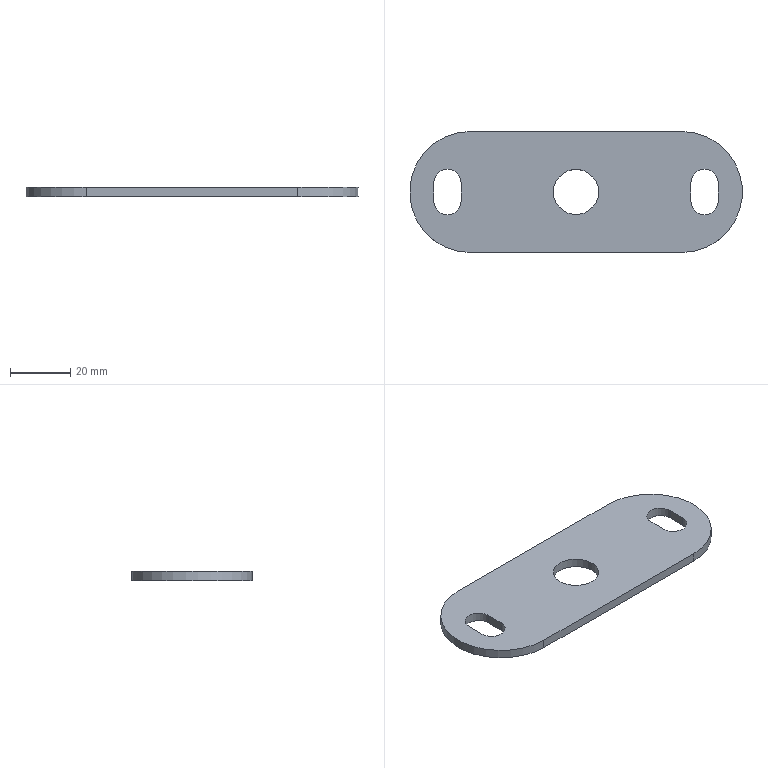Part | STEP file | PN_0011_default | 1 solid | 15 faces | box 110 x 40 x 3 mm | volume 10934 mm3 | plane 8 | cylinder 7 | commonest cylinder face diameters 9 x4 40 x2 15 x1
STEP:
#1=CARTESIAN_POINT('',(0.,0.,0.));
#2=DIRECTION('',(0.,0.,1.));
#3=DIRECTION('',(1.,0.,0.));
#4=AXIS2_PLACEMENT_3D('',#1,#2,#3);
#5=CARTESIAN_POINT('',(7.5,0.,3.));
#6=VERTEX_POINT('',#5);
#7=CARTESIAN_POINT('',(0.,0.,3.));
#8=DIRECTION('',(0.,0.,1.));
#9=DIRECTION('',(1.,0.,0.));
#10=AXIS2_PLACEMENT_3D('',#7,#8,#9);
#11=CIRCLE('',#10,7.5);
#12=CARTESIAN_POINT('',(-35.,0.,3.));
#13=DIRECTION('',(0.,0.,1.));
#14=DIRECTION('',(1.,0.,0.));
#15=AXIS2_PLACEMENT_3D('',#12,#13,#14);
#16=PLANE('',#15);
#17=CARTESIAN_POINT('',(35.,0.));
#18=DIRECTION('',(1.,0.));
#19=AXIS2_PLACEMENT_2D('',#17,#18);
#20=CIRCLE('',#19,7.5);
#21=(GEOMETRIC_REPRESENTATION_CONTEXT(2)PARAMETRIC_REPRESENTATION_CONTEXT()REPRESENTATION_CONTEXT('',''));
#22=DEFINITIONAL_REPRESENTATION('',(#20),#21);
#23=PCURVE('',#16,#22);
#24=CARTESIAN_POINT('',(0.,0.,-7.));
#25=DIRECTION('',(0.,0.,1.));
#26=DIRECTION('',(1.,0.,0.));
#27=AXIS2_PLACEMENT_3D('',#24,#25,#26);
#28=CYLINDRICAL_SURFACE('',#27,7.5);
#29=CARTESIAN_POINT('',(0.,10.));
#30=DIRECTION('',(1.,0.));
#31=VECTOR('',#30,1.);
#32=LINE('',#29,#31);
#33=(GEOMETRIC_REPRESENTATION_CONTEXT(2)PARAMETRIC_REPRESENTATION_CONTEXT()REPRESENTATION_CONTEXT('',''));
#34=DEFINITIONAL_REPRESENTATION('',(#32),#33);
#35=PCURVE('',#28,#34);
#36=SURFACE_CURVE('',#11,(#23,#35),.PCURVE_S1.);
#37=EDGE_CURVE('',#6,#6,#36,.T.);
#38=ORIENTED_EDGE('',*,*,#37,.F.);
#39=EDGE_LOOP('',(#38));
#40=FACE_BOUND('',#39,.T.);
#41=CARTESIAN_POINT('',(-47.,3.,3.));
#42=VERTEX_POINT('',#41);
#43=CARTESIAN_POINT('',(-47.,-3.,3.));
#44=VERTEX_POINT('',#43);
#45=CARTESIAN_POINT('',(-47.,3.,3.));
#46=DIRECTION('',(0.,-1.,0.));
#47=VECTOR('',#46,1.);
#48=LINE('',#45,#47);
#49=CARTESIAN_POINT('',(-12.,3.));
#50=DIRECTION('',(0.,-1.));
#51=VECTOR('',#50,1.);
#52=LINE('',#49,#51);
#53=(GEOMETRIC_REPRESENTATION_CONTEXT(2)PARAMETRIC_REPRESENTATION_CONTEXT()REPRESENTATION_CONTEXT('',''));
#54=DEFINITIONAL_REPRESENTATION('',(#52),#53);
#55=PCURVE('',#16,#54);
#56=CARTESIAN_POINT('',(-47.,3.,3.));
#57=DIRECTION('',(1.,0.,0.));
#58=DIRECTION('',(0.,0.,-1.));
#59=AXIS2_PLACEMENT_3D('',#56,#57,#58);
#60=PLANE('',#59);
#61=CARTESIAN_POINT('',(0.,0.));
#62=DIRECTION('',(0.,-1.));
#63=VECTOR('',#62,1.);
#64=LINE('',#61,#63);
#65=(GEOMETRIC_REPRESENTATION_CONTEXT(2)PARAMETRIC_REPRESENTATION_CONTEXT()REPRESENTATION_CONTEXT('',''));
#66=DEFINITIONAL_REPRESENTATION('',(#64),#65);
#67=PCURVE('',#60,#66);
#68=SURFACE_CURVE('',#48,(#55,#67),.PCURVE_S1.);
#69=EDGE_CURVE('',#42,#44,#68,.T.);
#70=ORIENTED_EDGE('',*,*,#69,.F.);
#71=CARTESIAN_POINT('',(-38.,3.,3.));
#72=VERTEX_POINT('',#71);
#73=CARTESIAN_POINT('',(-42.5,3.,3.));
#74=DIRECTION('',(0.,0.,1.));
#75=DIRECTION('',(1.,0.,0.));
#76=AXIS2_PLACEMENT_3D('',#73,#74,#75);
#77=CIRCLE('',#76,4.5);
#78=CARTESIAN_POINT('',(-7.5,3.));
#79=DIRECTION('',(1.,0.));
#80=AXIS2_PLACEMENT_2D('',#78,#79);
#81=CIRCLE('',#80,4.5);
#82=(GEOMETRIC_REPRESENTATION_CONTEXT(2)PARAMETRIC_REPRESENTATION_CONTEXT()REPRESENTATION_CONTEXT('',''));
#83=DEFINITIONAL_REPRESENTATION('',(#81),#82);
#84=PCURVE('',#16,#83);
#85=CARTESIAN_POINT('',(-42.5,3.,3.));
#86=DIRECTION('',(0.,0.,-1.));
#87=DIRECTION('',(-1.,0.,0.));
#88=AXIS2_PLACEMENT_3D('',#85,#86,#87);
#89=CYLINDRICAL_SURFACE('',#88,4.5);
#90=CARTESIAN_POINT('',(3.142,0.));
#91=DIRECTION('',(-1.,0.));
#92=VECTOR('',#91,1.);
#93=LINE('',#90,#92);
#94=(GEOMETRIC_REPRESENTATION_CONTEXT(2)PARAMETRIC_REPRESENTATION_CONTEXT()REPRESENTATION_CONTEXT('',''));
#95=DEFINITIONAL_REPRESENTATION('',(#93),#94);
#96=PCURVE('',#89,#95);
#97=SURFACE_CURVE('',#77,(#84,#96),.PCURVE_S1.);
#98=EDGE_CURVE('',#72,#42,#97,.T.);
#99=ORIENTED_EDGE('',*,*,#98,.F.);
#100=CARTESIAN_POINT('',(-38.,-3.,3.));
#101=VERTEX_POINT('',#100);
#102=CARTESIAN_POINT('',(-38.,3.,3.));
#103=DIRECTION('',(0.,1.,0.));
#104=VECTOR('',#103,1.);
#105=LINE('',#102,#104);
#106=CARTESIAN_POINT('',(-3.,3.));
#107=DIRECTION('',(0.,1.));
#108=VECTOR('',#107,1.);
#109=LINE('',#106,#108);
#110=(GEOMETRIC_REPRESENTATION_CONTEXT(2)PARAMETRIC_REPRESENTATION_CONTEXT()REPRESENTATION_CONTEXT('',''));
#111=DEFINITIONAL_REPRESENTATION('',(#109),#110);
#112=PCURVE('',#16,#111);
#113=CARTESIAN_POINT('',(-38.,3.,3.));
#114=DIRECTION('',(-1.,0.,0.));
#115=DIRECTION('',(0.,0.,1.));
#116=AXIS2_PLACEMENT_3D('',#113,#114,#115);
#117=PLANE('',#116);
#118=CARTESIAN_POINT('',(0.,0.));
#119=DIRECTION('',(0.,1.));
#120=VECTOR('',#119,1.);
#121=LINE('',#118,#120);
#122=(GEOMETRIC_REPRESENTATION_CONTEXT(2)PARAMETRIC_REPRESENTATION_CONTEXT()REPRESENTATION_CONTEXT('',''));
#123=DEFINITIONAL_REPRESENTATION('',(#121),#122);
#124=PCURVE('',#117,#123);
#125=SURFACE_CURVE('',#105,(#112,#124),.PCURVE_S1.);
#126=EDGE_CURVE('',#101,#72,#125,.T.);
#127=ORIENTED_EDGE('',*,*,#126,.F.);
#128=CARTESIAN_POINT('',(-42.5,-3.,3.));
#129=DIRECTION('',(0.,0.,1.));
#130=DIRECTION('',(1.,0.,0.));
#131=AXIS2_PLACEMENT_3D('',#128,#129,#130);
#132=CIRCLE('',#131,4.5);
#133=CARTESIAN_POINT('',(-7.5,-3.));
#134=DIRECTION('',(1.,0.));
#135=AXIS2_PLACEMENT_2D('',#133,#134);
#136=CIRCLE('',#135,4.5);
#137=(GEOMETRIC_REPRESENTATION_CONTEXT(2)PARAMETRIC_REPRESENTATION_CONTEXT()REPRESENTATION_CONTEXT('',''));
#138=DEFINITIONAL_REPRESENTATION('',(#136),#137);
#139=PCURVE('',#16,#138);
#140=CARTESIAN_POINT('',(-42.5,-3.,3.));
#141=DIRECTION('',(0.,0.,-1.));
#142=DIRECTION('',(-1.,0.,0.));
#143=AXIS2_PLACEMENT_3D('',#140,#141,#142);
#144=CYLINDRICAL_SURFACE('',#143,4.5);
#145=CARTESIAN_POINT('',(9.425,0.));
#146=DIRECTION('',(-1.,0.));
#147=VECTOR('',#146,1.);
#148=LINE('',#145,#147);
#149=(GEOMETRIC_REPRESENTATION_CONTEXT(2)PARAMETRIC_REPRESENTATION_CONTEXT()REPRESENTATION_CONTEXT('',''));
#150=DEFINITIONAL_REPRESENTATION('',(#148),#149);
#151=PCURVE('',#144,#150);
#152=SURFACE_CURVE('',#132,(#139,#151),.PCURVE_S1.);
#153=EDGE_CURVE('',#44,#101,#152,.T.);
#154=ORIENTED_EDGE('',*,*,#153,.F.);
#155=EDGE_LOOP('',(#70,#99,#127,#154));
#156=FACE_BOUND('',#155,.T.);
#157=CARTESIAN_POINT('',(-35.,20.,3.));
#158=VERTEX_POINT('',#157);
#159=CARTESIAN_POINT('',(-35.,-20.,3.));
#160=VERTEX_POINT('',#159);
#161=CARTESIAN_POINT('',(-35.,0.,3.));
#162=DIRECTION('',(0.,0.,1.));
#163=DIRECTION('',(1.,0.,0.));
#164=AXIS2_PLACEMENT_3D('',#161,#162,#163);
#165=CIRCLE('',#164,20.);
#166=CARTESIAN_POINT('',(0.,0.));
#167=DIRECTION('',(1.,0.));
#168=AXIS2_PLACEMENT_2D('',#166,#167);
#169=CIRCLE('',#168,20.);
#170=(GEOMETRIC_REPRESENTATION_CONTEXT(2)PARAMETRIC_REPRESENTATION_CONTEXT()REPRESENTATION_CONTEXT('',''));
#171=DEFINITIONAL_REPRESENTATION('',(#169),#170);
#172=PCURVE('',#16,#171);
#173=CARTESIAN_POINT('',(-35.,0.,3.));
#174=DIRECTION('',(0.,0.,-1.));
#175=DIRECTION('',(-1.,0.,0.));
#176=AXIS2_PLACEMENT_3D('',#173,#174,#175);
#177=CYLINDRICAL_SURFACE('',#176,20.);
#178=CARTESIAN_POINT('',(3.142,0.));
#179=DIRECTION('',(-1.,0.));
#180=VECTOR('',#179,1.);
#181=LINE('',#178,#180);
#182=(GEOMETRIC_REPRESENTATION_CONTEXT(2)PARAMETRIC_REPRESENTATION_CONTEXT()REPRESENTATION_CONTEXT('',''));
#183=DEFINITIONAL_REPRESENTATION('',(#181),#182);
#184=PCURVE('',#177,#183);
#185=SURFACE_CURVE('',#165,(#172,#184),.PCURVE_S1.);
#186=EDGE_CURVE('',#158,#160,#185,.T.);
#187=ORIENTED_EDGE('',*,*,#186,.T.);
#188=CARTESIAN_POINT('',(35.,-20.,3.));
#189=VERTEX_POINT('',#188);
#190=CARTESIAN_POINT('',(-35.,-20.,3.));
#191=DIRECTION('',(1.,0.,0.));
#192=VECTOR('',#191,1.);
#193=LINE('',#190,#192);
#194=CARTESIAN_POINT('',(0.,-20.));
#195=DIRECTION('',(1.,0.));
#196=VECTOR('',#195,1.);
#197=LINE('',#194,#196);
#198=(GEOMETRIC_REPRESENTATION_CONTEXT(2)PARAMETRIC_REPRESENTATION_CONTEXT()REPRESENTATION_CONTEXT('',''));
#199=DEFINITIONAL_REPRESENTATION('',(#197),#198);
#200=PCURVE('',#16,#199);
#201=CARTESIAN_POINT('',(-35.,-20.,3.));
#202=DIRECTION('',(0.,1.,0.));
#203=DIRECTION('',(0.,0.,1.));
#204=AXIS2_PLACEMENT_3D('',#201,#202,#203);
#205=PLANE('',#204);
#206=CARTESIAN_POINT('',(0.,0.));
#207=DIRECTION('',(0.,1.));
#208=VECTOR('',#207,1.);
#209=LINE('',#206,#208);
#210=(GEOMETRIC_REPRESENTATION_CONTEXT(2)PARAMETRIC_REPRESENTATION_CONTEXT()REPRESENTATION_CONTEXT('',''));
#211=DEFINITIONAL_REPRESENTATION('',(#209),#210);
#212=PCURVE('',#205,#211);
#213=SURFACE_CURVE('',#193,(#200,#212),.PCURVE_S1.);
#214=EDGE_CURVE('',#160,#189,#213,.T.);
#215=ORIENTED_EDGE('',*,*,#214,.T.);
#216=CARTESIAN_POINT('',(35.,20.,3.));
#217=VERTEX_POINT('',#216);
#218=CARTESIAN_POINT('',(35.,0.,3.));
#219=DIRECTION('',(0.,0.,1.));
#220=DIRECTION('',(-1.,0.,0.));
#221=AXIS2_PLACEMENT_3D('',#218,#219,#220);
#222=CIRCLE('',#221,20.);
#223=CARTESIAN_POINT('',(70.,0.));
#224=DIRECTION('',(-1.,0.));
#225=AXIS2_PLACEMENT_2D('',#223,#224);
#226=CIRCLE('',#225,20.);
#227=(GEOMETRIC_REPRESENTATION_CONTEXT(2)PARAMETRIC_REPRESENTATION_CONTEXT()REPRESENTATION_CONTEXT('',''));
#228=DEFINITIONAL_REPRESENTATION('',(#226),#227);
#229=PCURVE('',#16,#228);
#230=CARTESIAN_POINT('',(35.,0.,3.));
#231=DIRECTION('',(0.,0.,-1.));
#232=DIRECTION('',(-1.,0.,0.));
#233=AXIS2_PLACEMENT_3D('',#230,#231,#232);
#234=CYLINDRICAL_SURFACE('',#233,20.);
#235=CARTESIAN_POINT('',(6.283,0.));
#236=DIRECTION('',(-1.,0.));
#237=VECTOR('',#236,1.);
#238=LINE('',#235,#237);
#239=(GEOMETRIC_REPRESENTATION_CONTEXT(2)PARAMETRIC_REPRESENTATION_CONTEXT()REPRESENTATION_CONTEXT('',''));
#240=DEFINITIONAL_REPRESENTATION('',(#238),#239);
#241=PCURVE('',#234,#240);
#242=SURFACE_CURVE('',#222,(#229,#241),.PCURVE_S1.);
#243=EDGE_CURVE('',#189,#217,#242,.T.);
#244=ORIENTED_EDGE('',*,*,#243,.T.);
#245=CARTESIAN_POINT('',(-35.,20.,3.));
#246=DIRECTION('',(-1.,0.,0.));
#247=VECTOR('',#246,1.);
#248=LINE('',#245,#247);
#249=CARTESIAN_POINT('',(0.,20.));
#250=DIRECTION('',(-1.,0.));
#251=VECTOR('',#250,1.);
#252=LINE('',#249,#251);
#253=(GEOMETRIC_REPRESENTATION_CONTEXT(2)PARAMETRIC_REPRESENTATION_CONTEXT()REPRESENTATION_CONTEXT('',''));
#254=DEFINITIONAL_REPRESENTATION('',(#252),#253);
#255=PCURVE('',#16,#254);
#256=CARTESIAN_POINT('',(-35.,20.,3.));
#257=DIRECTION('',(0.,-1.,0.));
#258=DIRECTION('',(0.,0.,-1.));
#259=AXIS2_PLACEMENT_3D('',#256,#257,#258);
#260=PLANE('',#259);
#261=CARTESIAN_POINT('',(0.,0.));
#262=DIRECTION('',(0.,-1.));
#263=VECTOR('',#262,1.);
#264=LINE('',#261,#263);
#265=(GEOMETRIC_REPRESENTATION_CONTEXT(2)PARAMETRIC_REPRESENTATION_CONTEXT()REPRESENTATION_CONTEXT('',''));
#266=DEFINITIONAL_REPRESENTATION('',(#264),#265);
#267=PCURVE('',#260,#266);
#268=SURFACE_CURVE('',#248,(#255,#267),.PCURVE_S1.);
#269=EDGE_CURVE('',#217,#158,#268,.T.);
#270=ORIENTED_EDGE('',*,*,#269,.T.);
#271=EDGE_LOOP('',(#187,#215,#244,#270));
#272=FACE_BOUND('',#271,.T.);
#273=CARTESIAN_POINT('',(47.,-3.,3.));
#274=VERTEX_POINT('',#273);
#275=CARTESIAN_POINT('',(47.,3.,3.));
#276=VERTEX_POINT('',#275);
#277=CARTESIAN_POINT('',(47.,3.,3.));
#278=DIRECTION('',(0.,1.,0.));
#279=VECTOR('',#278,1.);
#280=LINE('',#277,#279);
#281=CARTESIAN_POINT('',(82.,3.));
#282=DIRECTION('',(0.,1.));
#283=VECTOR('',#282,1.);
#284=LINE('',#281,#283);
#285=(GEOMETRIC_REPRESENTATION_CONTEXT(2)PARAMETRIC_REPRESENTATION_CONTEXT()REPRESENTATION_CONTEXT('',''));
#286=DEFINITIONAL_REPRESENTATION('',(#284),#285);
#287=PCURVE('',#16,#286);
#288=CARTESIAN_POINT('',(47.,3.,3.));
#289=DIRECTION('',(-1.,0.,0.));
#290=DIRECTION('',(0.,0.,1.));
#291=AXIS2_PLACEMENT_3D('',#288,#289,#290);
#292=PLANE('',#291);
#293=CARTESIAN_POINT('',(0.,0.));
#294=DIRECTION('',(0.,1.));
#295=VECTOR('',#294,1.);
#296=LINE('',#293,#295);
#297=(GEOMETRIC_REPRESENTATION_CONTEXT(2)PARAMETRIC_REPRESENTATION_CONTEXT()REPRESENTATION_CONTEXT('',''));
#298=DEFINITIONAL_REPRESENTATION('',(#296),#297);
#299=PCURVE('',#292,#298);
#300=SURFACE_CURVE('',#280,(#287,#299),.PCURVE_S1.);
#301=EDGE_CURVE('',#274,#276,#300,.T.);
#302=ORIENTED_EDGE('',*,*,#301,.F.);
#303=CARTESIAN_POINT('',(38.,-3.,3.));
#304=VERTEX_POINT('',#303);
#305=CARTESIAN_POINT('',(42.5,-3.,3.));
#306=DIRECTION('',(0.,0.,1.));
#307=DIRECTION('',(1.,0.,0.));
#308=AXIS2_PLACEMENT_3D('',#305,#306,#307);
#309=CIRCLE('',#308,4.5);
#310=CARTESIAN_POINT('',(77.5,-3.));
#311=DIRECTION('',(1.,0.));
#312=AXIS2_PLACEMENT_2D('',#310,#311);
#313=CIRCLE('',#312,4.5);
#314=(GEOMETRIC_REPRESENTATION_CONTEXT(2)PARAMETRIC_REPRESENTATION_CONTEXT()REPRESENTATION_CONTEXT('',''));
#315=DEFINITIONAL_REPRESENTATION('',(#313),#314);
#316=PCURVE('',#16,#315);
#317=CARTESIAN_POINT('',(42.5,-3.,3.));
#318=DIRECTION('',(0.,0.,-1.));
#319=DIRECTION('',(-1.,0.,0.));
#320=AXIS2_PLACEMENT_3D('',#317,#318,#319);
#321=CYLINDRICAL_SURFACE('',#320,4.5);
#322=CARTESIAN_POINT('',(9.425,0.));
#323=DIRECTION('',(-1.,0.));
#324=VECTOR('',#323,1.);
#325=LINE('',#322,#324);
#326=(GEOMETRIC_REPRESENTATION_CONTEXT(2)PARAMETRIC_REPRESENTATION_CONTEXT()REPRESENTATION_CONTEXT('',''));
#327=DEFINITIONAL_REPRESENTATION('',(#325),#326);
#328=PCURVE('',#321,#327);
#329=SURFACE_CURVE('',#309,(#316,#328),.PCURVE_S1.);
#330=EDGE_CURVE('',#304,#274,#329,.T.);
#331=ORIENTED_EDGE('',*,*,#330,.F.);
#332=CARTESIAN_POINT('',(38.,3.,3.));
#333=VERTEX_POINT('',#332);
#334=CARTESIAN_POINT('',(38.,3.,3.));
#335=DIRECTION('',(0.,-1.,0.));
#336=VECTOR('',#335,1.);
#337=LINE('',#334,#336);
#338=CARTESIAN_POINT('',(73.,3.));
#339=DIRECTION('',(0.,-1.));
#340=VECTOR('',#339,1.);
#341=LINE('',#338,#340);
#342=(GEOMETRIC_REPRESENTATION_CONTEXT(2)PARAMETRIC_REPRESENTATION_CONTEXT()REPRESENTATION_CONTEXT('',''));
#343=DEFINITIONAL_REPRESENTATION('',(#341),#342);
#344=PCURVE('',#16,#343);
#345=CARTESIAN_POINT('',(38.,3.,3.));
#346=DIRECTION('',(1.,0.,0.));
#347=DIRECTION('',(0.,0.,-1.));
#348=AXIS2_PLACEMENT_3D('',#345,#346,#347);
#349=PLANE('',#348);
#350=CARTESIAN_POINT('',(0.,0.));
#351=DIRECTION('',(0.,-1.));
#352=VECTOR('',#351,1.);
#353=LINE('',#350,#352);
#354=(GEOMETRIC_REPRESENTATION_CONTEXT(2)PARAMETRIC_REPRESENTATION_CONTEXT()REPRESENTATION_CONTEXT('',''));
#355=DEFINITIONAL_REPRESENTATION('',(#353),#354);
#356=PCURVE('',#349,#355);
#357=SURFACE_CURVE('',#337,(#344,#356),.PCURVE_S1.);
#358=EDGE_CURVE('',#333,#304,#357,.T.);
#359=ORIENTED_EDGE('',*,*,#358,.F.);
#360=CARTESIAN_POINT('',(42.5,3.,3.));
#361=DIRECTION('',(0.,0.,1.));
#362=DIRECTION('',(1.,0.,0.));
#363=AXIS2_PLACEMENT_3D('',#360,#361,#362);
#364=CIRCLE('',#363,4.5);
#365=CARTESIAN_POINT('',(77.5,3.));
#366=DIRECTION('',(1.,0.));
#367=AXIS2_PLACEMENT_2D('',#365,#366);
#368=CIRCLE('',#367,4.5);
#369=(GEOMETRIC_REPRESENTATION_CONTEXT(2)PARAMETRIC_REPRESENTATION_CONTEXT()REPRESENTATION_CONTEXT('',''));
#370=DEFINITIONAL_REPRESENTATION('',(#368),#369);
#371=PCURVE('',#16,#370);
#372=CARTESIAN_POINT('',(42.5,3.,3.));
#373=DIRECTION('',(0.,0.,-1.));
#374=DIRECTION('',(-1.,0.,0.));
#375=AXIS2_PLACEMENT_3D('',#372,#373,#374);
#376=CYLINDRICAL_SURFACE('',#375,4.5);
#377=CARTESIAN_POINT('',(3.142,0.));
#378=DIRECTION('',(-1.,0.));
#379=VECTOR('',#378,1.);
#380=LINE('',#377,#379);
#381=(GEOMETRIC_REPRESENTATION_CONTEXT(2)PARAMETRIC_REPRESENTATION_CONTEXT()REPRESENTATION_CONTEXT('',''));
#382=DEFINITIONAL_REPRESENTATION('',(#380),#381);
#383=PCURVE('',#376,#382);
#384=SURFACE_CURVE('',#364,(#371,#383),.PCURVE_S1.);
#385=EDGE_CURVE('',#276,#333,#384,.T.);
#386=ORIENTED_EDGE('',*,*,#385,.F.);
#387=EDGE_LOOP('',(#302,#331,#359,#386));
#388=FACE_BOUND('',#387,.T.);
#389=ADVANCED_FACE('',(#40,#156,#272,#388),#16,.T.);
#390=CARTESIAN_POINT('',(7.5,0.,0.));
#391=VERTEX_POINT('',#390);
#392=CARTESIAN_POINT('',(0.,0.,0.));
#393=DIRECTION('',(0.,0.,1.));
#394=DIRECTION('',(1.,0.,0.));
#395=AXIS2_PLACEMENT_3D('',#392,#393,#394);
#396=CIRCLE('',#395,7.5);
#397=CARTESIAN_POINT('',(-35.,0.,0.));
#398=DIRECTION('',(0.,0.,1.));
#399=DIRECTION('',(1.,0.,0.));
#400=AXIS2_PLACEMENT_3D('',#397,#398,#399);
#401=PLANE('',#400);
#402=CARTESIAN_POINT('',(35.,0.));
#403=DIRECTION('',(1.,0.));
#404=AXIS2_PLACEMENT_2D('',#402,#403);
#405=CIRCLE('',#404,7.5);
#406=(GEOMETRIC_REPRESENTATION_CONTEXT(2)PARAMETRIC_REPRESENTATION_CONTEXT()REPRESENTATION_CONTEXT('',''));
#407=DEFINITIONAL_REPRESENTATION('',(#405),#406);
#408=PCURVE('',#401,#407);
#409=CARTESIAN_POINT('',(0.,7.));
#410=DIRECTION('',(1.,0.));
#411=VECTOR('',#410,1.);
#412=LINE('',#409,#411);
#413=(GEOMETRIC_REPRESENTATION_CONTEXT(2)PARAMETRIC_REPRESENTATION_CONTEXT()REPRESENTATION_CONTEXT('',''));
#414=DEFINITIONAL_REPRESENTATION('',(#412),#413);
#415=PCURVE('',#28,#414);
#416=SURFACE_CURVE('',#396,(#408,#415),.PCURVE_S1.);
#417=EDGE_CURVE('',#391,#391,#416,.T.);
#418=ORIENTED_EDGE('',*,*,#417,.T.);
#419=EDGE_LOOP('',(#418));
#420=FACE_BOUND('',#419,.T.);
#421=CARTESIAN_POINT('',(-38.,3.,0.));
#422=VERTEX_POINT('',#421);
#423=CARTESIAN_POINT('',(-47.,3.,0.));
#424=VERTEX_POINT('',#423);
#425=CARTESIAN_POINT('',(-42.5,3.,0.));
#426=DIRECTION('',(0.,0.,1.));
#427=DIRECTION('',(1.,0.,0.));
#428=AXIS2_PLACEMENT_3D('',#425,#426,#427);
#429=CIRCLE('',#428,4.5);
#430=CARTESIAN_POINT('',(-7.5,3.));
#431=DIRECTION('',(1.,0.));
#432=AXIS2_PLACEMENT_2D('',#430,#431);
#433=CIRCLE('',#432,4.5);
#434=(GEOMETRIC_REPRESENTATION_CONTEXT(2)PARAMETRIC_REPRESENTATION_CONTEXT()REPRESENTATION_CONTEXT('',''));
#435=DEFINITIONAL_REPRESENTATION('',(#433),#434);
#436=PCURVE('',#401,#435);
#437=CARTESIAN_POINT('',(3.142,3.));
#438=DIRECTION('',(-1.,0.));
#439=VECTOR('',#438,1.);
#440=LINE('',#437,#439);
#441=(GEOMETRIC_REPRESENTATION_CONTEXT(2)PARAMETRIC_REPRESENTATION_CONTEXT()REPRESENTATION_CONTEXT('',''));
#442=DEFINITIONAL_REPRESENTATION('',(#440),#441);
#443=PCURVE('',#89,#442);
#444=SURFACE_CURVE('',#429,(#436,#443),.PCURVE_S1.);
#445=EDGE_CURVE('',#422,#424,#444,.T.);
#446=ORIENTED_EDGE('',*,*,#445,.T.);
#447=CARTESIAN_POINT('',(-47.,-3.,0.));
#448=VERTEX_POINT('',#447);
#449=CARTESIAN_POINT('',(-47.,3.,0.));
#450=DIRECTION('',(0.,-1.,0.));
#451=VECTOR('',#450,1.);
#452=LINE('',#449,#451);
#453=CARTESIAN_POINT('',(-12.,3.));
#454=DIRECTION('',(0.,-1.));
#455=VECTOR('',#454,1.);
#456=LINE('',#453,#455);
#457=(GEOMETRIC_REPRESENTATION_CONTEXT(2)PARAMETRIC_REPRESENTATION_CONTEXT()REPRESENTATION_CONTEXT('',''));
#458=DEFINITIONAL_REPRESENTATION('',(#456),#457);
#459=PCURVE('',#401,#458);
#460=CARTESIAN_POINT('',(3.,0.));
#461=DIRECTION('',(0.,-1.));
#462=VECTOR('',#461,1.);
#463=LINE('',#460,#462);
#464=(GEOMETRIC_REPRESENTATION_CONTEXT(2)PARAMETRIC_REPRESENTATION_CONTEXT()REPRESENTATION_CONTEXT('',''));
#465=DEFINITIONAL_REPRESENTATION('',(#463),#464);
#466=PCURVE('',#60,#465);
#467=SURFACE_CURVE('',#452,(#459,#466),.PCURVE_S1.);
#468=EDGE_CURVE('',#424,#448,#467,.T.);
#469=ORIENTED_EDGE('',*,*,#468,.T.);
#470=CARTESIAN_POINT('',(-38.,-3.,0.));
#471=VERTEX_POINT('',#470);
#472=CARTESIAN_POINT('',(-42.5,-3.,0.));
#473=DIRECTION('',(0.,0.,1.));
#474=DIRECTION('',(1.,0.,0.));
#475=AXIS2_PLACEMENT_3D('',#472,#473,#474);
#476=CIRCLE('',#475,4.5);
#477=CARTESIAN_POINT('',(-7.5,-3.));
#478=DIRECTION('',(1.,0.));
#479=AXIS2_PLACEMENT_2D('',#477,#478);
#480=CIRCLE('',#479,4.5);
#481=(GEOMETRIC_REPRESENTATION_CONTEXT(2)PARAMETRIC_REPRESENTATION_CONTEXT()REPRESENTATION_CONTEXT('',''));
#482=DEFINITIONAL_REPRESENTATION('',(#480),#481);
#483=PCURVE('',#401,#482);
#484=CARTESIAN_POINT('',(9.425,3.));
#485=DIRECTION('',(-1.,0.));
#486=VECTOR('',#485,1.);
#487=LINE('',#484,#486);
#488=(GEOMETRIC_REPRESENTATION_CONTEXT(2)PARAMETRIC_REPRESENTATION_CONTEXT()REPRESENTATION_CONTEXT('',''));
#489=DEFINITIONAL_REPRESENTATION('',(#487),#488);
#490=PCURVE('',#144,#489);
#491=SURFACE_CURVE('',#476,(#483,#490),.PCURVE_S1.);
#492=EDGE_CURVE('',#448,#471,#491,.T.);
#493=ORIENTED_EDGE('',*,*,#492,.T.);
#494=CARTESIAN_POINT('',(-38.,3.,0.));
#495=DIRECTION('',(0.,1.,0.));
#496=VECTOR('',#495,1.);
#497=LINE('',#494,#496);
#498=CARTESIAN_POINT('',(-3.,3.));
#499=DIRECTION('',(0.,1.));
#500=VECTOR('',#499,1.);
#501=LINE('',#498,#500);
#502=(GEOMETRIC_REPRESENTATION_CONTEXT(2)PARAMETRIC_REPRESENTATION_CONTEXT()REPRESENTATION_CONTEXT('',''));
#503=DEFINITIONAL_REPRESENTATION('',(#501),#502);
#504=PCURVE('',#401,#503);
#505=CARTESIAN_POINT('',(-3.,0.));
#506=DIRECTION('',(0.,1.));
#507=VECTOR('',#506,1.);
#508=LINE('',#505,#507);
#509=(GEOMETRIC_REPRESENTATION_CONTEXT(2)PARAMETRIC_REPRESENTATION_CONTEXT()REPRESENTATION_CONTEXT('',''));
#510=DEFINITIONAL_REPRESENTATION('',(#508),#509);
#511=PCURVE('',#117,#510);
#512=SURFACE_CURVE('',#497,(#504,#511),.PCURVE_S1.);
#513=EDGE_CURVE('',#471,#422,#512,.T.);
#514=ORIENTED_EDGE('',*,*,#513,.T.);
#515=EDGE_LOOP('',(#446,#469,#493,#514));
#516=FACE_BOUND('',#515,.T.);
#517=CARTESIAN_POINT('',(-35.,20.,0.));
#518=VERTEX_POINT('',#517);
#519=CARTESIAN_POINT('',(-35.,-20.,0.));
#520=VERTEX_POINT('',#519);
#521=CARTESIAN_POINT('',(-35.,0.,0.));
#522=DIRECTION('',(0.,0.,1.));
#523=DIRECTION('',(1.,0.,0.));
#524=AXIS2_PLACEMENT_3D('',#521,#522,#523);
#525=CIRCLE('',#524,20.);
#526=CARTESIAN_POINT('',(0.,0.));
#527=DIRECTION('',(1.,0.));
#528=AXIS2_PLACEMENT_2D('',#526,#527);
#529=CIRCLE('',#528,20.);
#530=(GEOMETRIC_REPRESENTATION_CONTEXT(2)PARAMETRIC_REPRESENTATION_CONTEXT()REPRESENTATION_CONTEXT('',''));
#531=DEFINITIONAL_REPRESENTATION('',(#529),#530);
#532=PCURVE('',#401,#531);
#533=CARTESIAN_POINT('',(3.142,3.));
#534=DIRECTION('',(-1.,0.));
#535=VECTOR('',#534,1.);
#536=LINE('',#533,#535);
#537=(GEOMETRIC_REPRESENTATION_CONTEXT(2)PARAMETRIC_REPRESENTATION_CONTEXT()REPRESENTATION_CONTEXT('',''));
#538=DEFINITIONAL_REPRESENTATION('',(#536),#537);
#539=PCURVE('',#177,#538);
#540=SURFACE_CURVE('',#525,(#532,#539),.PCURVE_S1.);
#541=EDGE_CURVE('',#518,#520,#540,.T.);
#542=ORIENTED_EDGE('',*,*,#541,.F.);
#543=CARTESIAN_POINT('',(35.,20.,0.));
#544=VERTEX_POINT('',#543);
#545=CARTESIAN_POINT('',(-35.,20.,0.));
#546=DIRECTION('',(-1.,0.,0.));
#547=VECTOR('',#546,1.);
#548=LINE('',#545,#547);
#549=CARTESIAN_POINT('',(0.,20.));
#550=DIRECTION('',(-1.,0.));
#551=VECTOR('',#550,1.);
#552=LINE('',#549,#551);
#553=(GEOMETRIC_REPRESENTATION_CONTEXT(2)PARAMETRIC_REPRESENTATION_CONTEXT()REPRESENTATION_CONTEXT('',''));
#554=DEFINITIONAL_REPRESENTATION('',(#552),#553);
#555=PCURVE('',#401,#554);
#556=CARTESIAN_POINT('',(3.,0.));
#557=DIRECTION('',(0.,-1.));
#558=VECTOR('',#557,1.);
#559=LINE('',#556,#558);
#560=(GEOMETRIC_REPRESENTATION_CONTEXT(2)PARAMETRIC_REPRESENTATION_CONTEXT()REPRESENTATION_CONTEXT('',''));
#561=DEFINITIONAL_REPRESENTATION('',(#559),#560);
#562=PCURVE('',#260,#561);
#563=SURFACE_CURVE('',#548,(#555,#562),.PCURVE_S1.);
#564=EDGE_CURVE('',#544,#518,#563,.T.);
#565=ORIENTED_EDGE('',*,*,#564,.F.);
#566=CARTESIAN_POINT('',(35.,-20.,0.));
#567=VERTEX_POINT('',#566);
#568=CARTESIAN_POINT('',(35.,0.,0.));
#569=DIRECTION('',(0.,0.,1.));
#570=DIRECTION('',(-1.,0.,0.));
#571=AXIS2_PLACEMENT_3D('',#568,#569,#570);
#572=CIRCLE('',#571,20.);
#573=CARTESIAN_POINT('',(70.,0.));
#574=DIRECTION('',(-1.,0.));
#575=AXIS2_PLACEMENT_2D('',#573,#574);
#576=CIRCLE('',#575,20.);
#577=(GEOMETRIC_REPRESENTATION_CONTEXT(2)PARAMETRIC_REPRESENTATION_CONTEXT()REPRESENTATION_CONTEXT('',''));
#578=DEFINITIONAL_REPRESENTATION('',(#576),#577);
#579=PCURVE('',#401,#578);
#580=CARTESIAN_POINT('',(6.283,3.));
#581=DIRECTION('',(-1.,0.));
#582=VECTOR('',#581,1.);
#583=LINE('',#580,#582);
#584=(GEOMETRIC_REPRESENTATION_CONTEXT(2)PARAMETRIC_REPRESENTATION_CONTEXT()REPRESENTATION_CONTEXT('',''));
#585=DEFINITIONAL_REPRESENTATION('',(#583),#584);
#586=PCURVE('',#234,#585);
#587=SURFACE_CURVE('',#572,(#579,#586),.PCURVE_S1.);
#588=EDGE_CURVE('',#567,#544,#587,.T.);
#589=ORIENTED_EDGE('',*,*,#588,.F.);
#590=CARTESIAN_POINT('',(-35.,-20.,0.));
#591=DIRECTION('',(1.,0.,0.));
#592=VECTOR('',#591,1.);
#593=LINE('',#590,#592);
#594=CARTESIAN_POINT('',(0.,-20.));
#595=DIRECTION('',(1.,0.));
#596=VECTOR('',#595,1.);
#597=LINE('',#594,#596);
#598=(GEOMETRIC_REPRESENTATION_CONTEXT(2)PARAMETRIC_REPRESENTATION_CONTEXT()REPRESENTATION_CONTEXT('',''));
#599=DEFINITIONAL_REPRESENTATION('',(#597),#598);
#600=PCURVE('',#401,#599);
#601=CARTESIAN_POINT('',(-3.,0.));
#602=DIRECTION('',(0.,1.));
#603=VECTOR('',#602,1.);
#604=LINE('',#601,#603);
#605=(GEOMETRIC_REPRESENTATION_CONTEXT(2)PARAMETRIC_REPRESENTATION_CONTEXT()REPRESENTATION_CONTEXT('',''));
#606=DEFINITIONAL_REPRESENTATION('',(#604),#605);
#607=PCURVE('',#205,#606);
#608=SURFACE_CURVE('',#593,(#600,#607),.PCURVE_S1.);
#609=EDGE_CURVE('',#520,#567,#608,.T.);
#610=ORIENTED_EDGE('',*,*,#609,.F.);
#611=EDGE_LOOP('',(#542,#565,#589,#610));
#612=FACE_BOUND('',#611,.T.);
#613=CARTESIAN_POINT('',(38.,-3.,0.));
#614=VERTEX_POINT('',#613);
#615=CARTESIAN_POINT('',(47.,-3.,0.));
#616=VERTEX_POINT('',#615);
#617=CARTESIAN_POINT('',(42.5,-3.,0.));
#618=DIRECTION('',(0.,0.,1.));
#619=DIRECTION('',(1.,0.,0.));
#620=AXIS2_PLACEMENT_3D('',#617,#618,#619);
#621=CIRCLE('',#620,4.5);
#622=CARTESIAN_POINT('',(77.5,-3.));
#623=DIRECTION('',(1.,0.));
#624=AXIS2_PLACEMENT_2D('',#622,#623);
#625=CIRCLE('',#624,4.5);
#626=(GEOMETRIC_REPRESENTATION_CONTEXT(2)PARAMETRIC_REPRESENTATION_CONTEXT()REPRESENTATION_CONTEXT('',''));
#627=DEFINITIONAL_REPRESENTATION('',(#625),#626);
#628=PCURVE('',#401,#627);
#629=CARTESIAN_POINT('',(9.425,3.));
#630=DIRECTION('',(-1.,0.));
#631=VECTOR('',#630,1.);
#632=LINE('',#629,#631);
#633=(GEOMETRIC_REPRESENTATION_CONTEXT(2)PARAMETRIC_REPRESENTATION_CONTEXT()REPRESENTATION_CONTEXT('',''));
#634=DEFINITIONAL_REPRESENTATION('',(#632),#633);
#635=PCURVE('',#321,#634);
#636=SURFACE_CURVE('',#621,(#628,#635),.PCURVE_S1.);
#637=EDGE_CURVE('',#614,#616,#636,.T.);
#638=ORIENTED_EDGE('',*,*,#637,.T.);
#639=CARTESIAN_POINT('',(47.,3.,0.));
#640=VERTEX_POINT('',#639);
#641=CARTESIAN_POINT('',(47.,3.,0.));
#642=DIRECTION('',(0.,1.,0.));
#643=VECTOR('',#642,1.);
#644=LINE('',#641,#643);
#645=CARTESIAN_POINT('',(82.,3.));
#646=DIRECTION('',(0.,1.));
#647=VECTOR('',#646,1.);
#648=LINE('',#645,#647);
#649=(GEOMETRIC_REPRESENTATION_CONTEXT(2)PARAMETRIC_REPRESENTATION_CONTEXT()REPRESENTATION_CONTEXT('',''));
#650=DEFINITIONAL_REPRESENTATION('',(#648),#649);
#651=PCURVE('',#401,#650);
#652=CARTESIAN_POINT('',(-3.,0.));
#653=DIRECTION('',(0.,1.));
#654=VECTOR('',#653,1.);
#655=LINE('',#652,#654);
#656=(GEOMETRIC_REPRESENTATION_CONTEXT(2)PARAMETRIC_REPRESENTATION_CONTEXT()REPRESENTATION_CONTEXT('',''));
#657=DEFINITIONAL_REPRESENTATION('',(#655),#656);
#658=PCURVE('',#292,#657);
#659=SURFACE_CURVE('',#644,(#651,#658),.PCURVE_S1.);
#660=EDGE_CURVE('',#616,#640,#659,.T.);
#661=ORIENTED_EDGE('',*,*,#660,.T.);
#662=CARTESIAN_POINT('',(38.,3.,0.));
#663=VERTEX_POINT('',#662);
#664=CARTESIAN_POINT('',(42.5,3.,0.));
#665=DIRECTION('',(0.,0.,1.));
#666=DIRECTION('',(1.,0.,0.));
#667=AXIS2_PLACEMENT_3D('',#664,#665,#666);
#668=CIRCLE('',#667,4.5);
#669=CARTESIAN_POINT('',(77.5,3.));
#670=DIRECTION('',(1.,0.));
#671=AXIS2_PLACEMENT_2D('',#669,#670);
#672=CIRCLE('',#671,4.5);
#673=(GEOMETRIC_REPRESENTATION_CONTEXT(2)PARAMETRIC_REPRESENTATION_CONTEXT()REPRESENTATION_CONTEXT('',''));
#674=DEFINITIONAL_REPRESENTATION('',(#672),#673);
#675=PCURVE('',#401,#674);
#676=CARTESIAN_POINT('',(3.142,3.));
#677=DIRECTION('',(-1.,0.));
#678=VECTOR('',#677,1.);
#679=LINE('',#676,#678);
#680=(GEOMETRIC_REPRESENTATION_CONTEXT(2)PARAMETRIC_REPRESENTATION_CONTEXT()REPRESENTATION_CONTEXT('',''));
#681=DEFINITIONAL_REPRESENTATION('',(#679),#680);
#682=PCURVE('',#376,#681);
#683=SURFACE_CURVE('',#668,(#675,#682),.PCURVE_S1.);
#684=EDGE_CURVE('',#640,#663,#683,.T.);
#685=ORIENTED_EDGE('',*,*,#684,.T.);
#686=CARTESIAN_POINT('',(38.,3.,0.));
#687=DIRECTION('',(0.,-1.,0.));
#688=VECTOR('',#687,1.);
#689=LINE('',#686,#688);
#690=CARTESIAN_POINT('',(73.,3.));
#691=DIRECTION('',(0.,-1.));
#692=VECTOR('',#691,1.);
#693=LINE('',#690,#692);
#694=(GEOMETRIC_REPRESENTATION_CONTEXT(2)PARAMETRIC_REPRESENTATION_CONTEXT()REPRESENTATION_CONTEXT('',''));
#695=DEFINITIONAL_REPRESENTATION('',(#693),#694);
#696=PCURVE('',#401,#695);
#697=CARTESIAN_POINT('',(3.,0.));
#698=DIRECTION('',(0.,-1.));
#699=VECTOR('',#698,1.);
#700=LINE('',#697,#699);
#701=(GEOMETRIC_REPRESENTATION_CONTEXT(2)PARAMETRIC_REPRESENTATION_CONTEXT()REPRESENTATION_CONTEXT('',''));
#702=DEFINITIONAL_REPRESENTATION('',(#700),#701);
#703=PCURVE('',#349,#702);
#704=SURFACE_CURVE('',#689,(#696,#703),.PCURVE_S1.);
#705=EDGE_CURVE('',#663,#614,#704,.T.);
#706=ORIENTED_EDGE('',*,*,#705,.T.);
#707=EDGE_LOOP('',(#638,#661,#685,#706));
#708=FACE_BOUND('',#707,.T.);
#709=ADVANCED_FACE('',(#420,#516,#612,#708),#401,.F.);
#710=ORIENTED_EDGE('',*,*,#541,.T.);
#711=CARTESIAN_POINT('',(-35.,-20.,3.));
#712=DIRECTION('',(0.,0.,-1.));
#713=VECTOR('',#712,1.);
#714=LINE('',#711,#713);
#715=CARTESIAN_POINT('',(-1.571,0.));
#716=DIRECTION('',(0.,1.));
#717=VECTOR('',#716,1.);
#718=LINE('',#715,#717);
#719=(GEOMETRIC_REPRESENTATION_CONTEXT(2)PARAMETRIC_REPRESENTATION_CONTEXT()REPRESENTATION_CONTEXT('',''));
#720=DEFINITIONAL_REPRESENTATION('',(#718),#719);
#721=PCURVE('',#177,#720);
#722=CARTESIAN_POINT('',(0.,0.));
#723=DIRECTION('',(-1.,0.));
#724=VECTOR('',#723,1.);
#725=LINE('',#722,#724);
#726=(GEOMETRIC_REPRESENTATION_CONTEXT(2)PARAMETRIC_REPRESENTATION_CONTEXT()REPRESENTATION_CONTEXT('',''));
#727=DEFINITIONAL_REPRESENTATION('',(#725),#726);
#728=PCURVE('',#205,#727);
#729=SURFACE_CURVE('',#714,(#721,#728),.PCURVE_S1.);
#730=EDGE_CURVE('',#160,#520,#729,.T.);
#731=ORIENTED_EDGE('',*,*,#730,.F.);
#732=ORIENTED_EDGE('',*,*,#186,.F.);
#733=CARTESIAN_POINT('',(-35.,20.,3.));
#734=DIRECTION('',(0.,0.,-1.));
#735=VECTOR('',#734,1.);
#736=LINE('',#733,#735);
#737=CARTESIAN_POINT('',(1.571,0.));
#738=DIRECTION('',(0.,1.));
#739=VECTOR('',#738,1.);
#740=LINE('',#737,#739);
#741=(GEOMETRIC_REPRESENTATION_CONTEXT(2)PARAMETRIC_REPRESENTATION_CONTEXT()REPRESENTATION_CONTEXT('',''));
#742=DEFINITIONAL_REPRESENTATION('',(#740),#741);
#743=PCURVE('',#177,#742);
#744=CARTESIAN_POINT('',(0.,0.));
#745=DIRECTION('',(1.,0.));
#746=VECTOR('',#745,1.);
#747=LINE('',#744,#746);
#748=(GEOMETRIC_REPRESENTATION_CONTEXT(2)PARAMETRIC_REPRESENTATION_CONTEXT()REPRESENTATION_CONTEXT('',''));
#749=DEFINITIONAL_REPRESENTATION('',(#747),#748);
#750=PCURVE('',#260,#749);
#751=SURFACE_CURVE('',#736,(#743,#750),.PCURVE_S1.);
#752=EDGE_CURVE('',#158,#518,#751,.T.);
#753=ORIENTED_EDGE('',*,*,#752,.T.);
#754=EDGE_LOOP('',(#710,#731,#732,#753));
#755=FACE_BOUND('',#754,.T.);
#756=ADVANCED_FACE('',(#755),#177,.T.);
#757=ORIENTED_EDGE('',*,*,#609,.T.);
#758=CARTESIAN_POINT('',(35.,-20.,3.));
#759=DIRECTION('',(0.,0.,-1.));
#760=VECTOR('',#759,1.);
#761=LINE('',#758,#760);
#762=CARTESIAN_POINT('',(0.,70.));
#763=DIRECTION('',(-1.,0.));
#764=VECTOR('',#763,1.);
#765=LINE('',#762,#764);
#766=(GEOMETRIC_REPRESENTATION_CONTEXT(2)PARAMETRIC_REPRESENTATION_CONTEXT()REPRESENTATION_CONTEXT('',''));
#767=DEFINITIONAL_REPRESENTATION('',(#765),#766);
#768=PCURVE('',#205,#767);
#769=CARTESIAN_POINT('',(4.712,0.));
#770=DIRECTION('',(0.,1.));
#771=VECTOR('',#770,1.);
#772=LINE('',#769,#771);
#773=(GEOMETRIC_REPRESENTATION_CONTEXT(2)PARAMETRIC_REPRESENTATION_CONTEXT()REPRESENTATION_CONTEXT('',''));
#774=DEFINITIONAL_REPRESENTATION('',(#772),#773);
#775=PCURVE('',#234,#774);
#776=SURFACE_CURVE('',#761,(#768,#775),.PCURVE_S1.);
#777=EDGE_CURVE('',#189,#567,#776,.T.);
#778=ORIENTED_EDGE('',*,*,#777,.F.);
#779=ORIENTED_EDGE('',*,*,#214,.F.);
#780=ORIENTED_EDGE('',*,*,#730,.T.);
#781=EDGE_LOOP('',(#757,#778,#779,#780));
#782=FACE_BOUND('',#781,.T.);
#783=ADVANCED_FACE('',(#782),#205,.F.);
#784=ORIENTED_EDGE('',*,*,#588,.T.);
#785=CARTESIAN_POINT('',(35.,20.,3.));
#786=DIRECTION('',(0.,0.,-1.));
#787=VECTOR('',#786,1.);
#788=LINE('',#785,#787);
#789=CARTESIAN_POINT('',(1.571,0.));
#790=DIRECTION('',(0.,1.));
#791=VECTOR('',#790,1.);
#792=LINE('',#789,#791);
#793=(GEOMETRIC_REPRESENTATION_CONTEXT(2)PARAMETRIC_REPRESENTATION_CONTEXT()REPRESENTATION_CONTEXT('',''));
#794=DEFINITIONAL_REPRESENTATION('',(#792),#793);
#795=PCURVE('',#234,#794);
#796=CARTESIAN_POINT('',(0.,70.));
#797=DIRECTION('',(1.,0.));
#798=VECTOR('',#797,1.);
#799=LINE('',#796,#798);
#800=(GEOMETRIC_REPRESENTATION_CONTEXT(2)PARAMETRIC_REPRESENTATION_CONTEXT()REPRESENTATION_CONTEXT('',''));
#801=DEFINITIONAL_REPRESENTATION('',(#799),#800);
#802=PCURVE('',#260,#801);
#803=SURFACE_CURVE('',#788,(#795,#802),.PCURVE_S1.);
#804=EDGE_CURVE('',#217,#544,#803,.T.);
#805=ORIENTED_EDGE('',*,*,#804,.F.);
#806=ORIENTED_EDGE('',*,*,#243,.F.);
#807=ORIENTED_EDGE('',*,*,#777,.T.);
#808=EDGE_LOOP('',(#784,#805,#806,#807));
#809=FACE_BOUND('',#808,.T.);
#810=ADVANCED_FACE('',(#809),#234,.T.);
#811=ORIENTED_EDGE('',*,*,#564,.T.);
#812=ORIENTED_EDGE('',*,*,#752,.F.);
#813=ORIENTED_EDGE('',*,*,#269,.F.);
#814=ORIENTED_EDGE('',*,*,#804,.T.);
#815=EDGE_LOOP('',(#811,#812,#813,#814));
#816=FACE_BOUND('',#815,.T.);
#817=ADVANCED_FACE('',(#816),#260,.F.);
#818=CARTESIAN_POINT('',(-47.,3.,3.));
#819=DIRECTION('',(0.,0.,-1.));
#820=VECTOR('',#819,1.);
#821=LINE('',#818,#820);
#822=CARTESIAN_POINT('',(0.,0.));
#823=DIRECTION('',(0.,1.));
#824=VECTOR('',#823,1.);
#825=LINE('',#822,#824);
#826=(GEOMETRIC_REPRESENTATION_CONTEXT(2)PARAMETRIC_REPRESENTATION_CONTEXT()REPRESENTATION_CONTEXT('',''));
#827=DEFINITIONAL_REPRESENTATION('',(#825),#826);
#828=PCURVE('',#89,#827);
#829=CARTESIAN_POINT('',(0.,0.));
#830=DIRECTION('',(1.,0.));
#831=VECTOR('',#830,1.);
#832=LINE('',#829,#831);
#833=(GEOMETRIC_REPRESENTATION_CONTEXT(2)PARAMETRIC_REPRESENTATION_CONTEXT()REPRESENTATION_CONTEXT('',''));
#834=DEFINITIONAL_REPRESENTATION('',(#832),#833);
#835=PCURVE('',#60,#834);
#836=SURFACE_CURVE('',#821,(#828,#835),.PCURVE_S1.);
#837=EDGE_CURVE('',#42,#424,#836,.T.);
#838=ORIENTED_EDGE('',*,*,#837,.F.);
#839=ORIENTED_EDGE('',*,*,#98,.F.);
#840=CARTESIAN_POINT('',(-38.,3.,3.));
#841=DIRECTION('',(0.,0.,-1.));
#842=VECTOR('',#841,1.);
#843=LINE('',#840,#842);
#844=CARTESIAN_POINT('',(3.142,0.));
#845=DIRECTION('',(0.,1.));
#846=VECTOR('',#845,1.);
#847=LINE('',#844,#846);
#848=(GEOMETRIC_REPRESENTATION_CONTEXT(2)PARAMETRIC_REPRESENTATION_CONTEXT()REPRESENTATION_CONTEXT('',''));
#849=DEFINITIONAL_REPRESENTATION('',(#847),#848);
#850=PCURVE('',#89,#849);
#851=CARTESIAN_POINT('',(0.,0.));
#852=DIRECTION('',(-1.,0.));
#853=VECTOR('',#852,1.);
#854=LINE('',#851,#853);
#855=(GEOMETRIC_REPRESENTATION_CONTEXT(2)PARAMETRIC_REPRESENTATION_CONTEXT()REPRESENTATION_CONTEXT('',''));
#856=DEFINITIONAL_REPRESENTATION('',(#854),#855);
#857=PCURVE('',#117,#856);
#858=SURFACE_CURVE('',#843,(#850,#857),.PCURVE_S1.);
#859=EDGE_CURVE('',#72,#422,#858,.T.);
#860=ORIENTED_EDGE('',*,*,#859,.T.);
#861=ORIENTED_EDGE('',*,*,#445,.T.);
#862=EDGE_LOOP('',(#838,#839,#860,#861));
#863=FACE_BOUND('',#862,.F.);
#864=ADVANCED_FACE('',(#863),#89,.F.);
#865=ORIENTED_EDGE('',*,*,#468,.F.);
#866=ORIENTED_EDGE('',*,*,#837,.F.);
#867=ORIENTED_EDGE('',*,*,#69,.T.);
#868=CARTESIAN_POINT('',(-47.,-3.,3.));
#869=DIRECTION('',(0.,0.,-1.));
#870=VECTOR('',#869,1.);
#871=LINE('',#868,#870);
#872=CARTESIAN_POINT('',(0.,-6.));
#873=DIRECTION('',(1.,0.));
#874=VECTOR('',#873,1.);
#875=LINE('',#872,#874);
#876=(GEOMETRIC_REPRESENTATION_CONTEXT(2)PARAMETRIC_REPRESENTATION_CONTEXT()REPRESENTATION_CONTEXT('',''));
#877=DEFINITIONAL_REPRESENTATION('',(#875),#876);
#878=PCURVE('',#60,#877);
#879=CARTESIAN_POINT('',(6.283,0.));
#880=DIRECTION('',(0.,1.));
#881=VECTOR('',#880,1.);
#882=LINE('',#879,#881);
#883=(GEOMETRIC_REPRESENTATION_CONTEXT(2)PARAMETRIC_REPRESENTATION_CONTEXT()REPRESENTATION_CONTEXT('',''));
#884=DEFINITIONAL_REPRESENTATION('',(#882),#883);
#885=PCURVE('',#144,#884);
#886=SURFACE_CURVE('',#871,(#878,#885),.PCURVE_S1.);
#887=EDGE_CURVE('',#44,#448,#886,.T.);
#888=ORIENTED_EDGE('',*,*,#887,.T.);
#889=EDGE_LOOP('',(#865,#866,#867,#888));
#890=FACE_BOUND('',#889,.T.);
#891=ADVANCED_FACE('',(#890),#60,.T.);
#892=CARTESIAN_POINT('',(-38.,-3.,3.));
#893=DIRECTION('',(0.,0.,-1.));
#894=VECTOR('',#893,1.);
#895=LINE('',#892,#894);
#896=CARTESIAN_POINT('',(3.142,0.));
#897=DIRECTION('',(0.,1.));
#898=VECTOR('',#897,1.);
#899=LINE('',#896,#898);
#900=(GEOMETRIC_REPRESENTATION_CONTEXT(2)PARAMETRIC_REPRESENTATION_CONTEXT()REPRESENTATION_CONTEXT('',''));
#901=DEFINITIONAL_REPRESENTATION('',(#899),#900);
#902=PCURVE('',#144,#901);
#903=CARTESIAN_POINT('',(0.,-6.));
#904=DIRECTION('',(-1.,0.));
#905=VECTOR('',#904,1.);
#906=LINE('',#903,#905);
#907=(GEOMETRIC_REPRESENTATION_CONTEXT(2)PARAMETRIC_REPRESENTATION_CONTEXT()REPRESENTATION_CONTEXT('',''));
#908=DEFINITIONAL_REPRESENTATION('',(#906),#907);
#909=PCURVE('',#117,#908);
#910=SURFACE_CURVE('',#895,(#902,#909),.PCURVE_S1.);
#911=EDGE_CURVE('',#101,#471,#910,.T.);
#912=ORIENTED_EDGE('',*,*,#911,.F.);
#913=ORIENTED_EDGE('',*,*,#153,.F.);
#914=ORIENTED_EDGE('',*,*,#887,.T.);
#915=ORIENTED_EDGE('',*,*,#492,.T.);
#916=EDGE_LOOP('',(#912,#913,#914,#915));
#917=FACE_BOUND('',#916,.F.);
#918=ADVANCED_FACE('',(#917),#144,.F.);
#919=ORIENTED_EDGE('',*,*,#513,.F.);
#920=ORIENTED_EDGE('',*,*,#911,.F.);
#921=ORIENTED_EDGE('',*,*,#126,.T.);
#922=ORIENTED_EDGE('',*,*,#859,.T.);
#923=EDGE_LOOP('',(#919,#920,#921,#922));
#924=FACE_BOUND('',#923,.T.);
#925=ADVANCED_FACE('',(#924),#117,.T.);
#926=CARTESIAN_POINT('',(47.,-3.,3.));
#927=DIRECTION('',(0.,0.,-1.));
#928=VECTOR('',#927,1.);
#929=LINE('',#926,#928);
#930=CARTESIAN_POINT('',(3.142,0.));
#931=DIRECTION('',(0.,1.));
#932=VECTOR('',#931,1.);
#933=LINE('',#930,#932);
#934=(GEOMETRIC_REPRESENTATION_CONTEXT(2)PARAMETRIC_REPRESENTATION_CONTEXT()REPRESENTATION_CONTEXT('',''));
#935=DEFINITIONAL_REPRESENTATION('',(#933),#934);
#936=PCURVE('',#321,#935);
#937=CARTESIAN_POINT('',(0.,-6.));
#938=DIRECTION('',(-1.,0.));
#939=VECTOR('',#938,1.);
#940=LINE('',#937,#939);
#941=(GEOMETRIC_REPRESENTATION_CONTEXT(2)PARAMETRIC_REPRESENTATION_CONTEXT()REPRESENTATION_CONTEXT('',''));
#942=DEFINITIONAL_REPRESENTATION('',(#940),#941);
#943=PCURVE('',#292,#942);
#944=SURFACE_CURVE('',#929,(#936,#943),.PCURVE_S1.);
#945=EDGE_CURVE('',#274,#616,#944,.T.);
#946=ORIENTED_EDGE('',*,*,#945,.F.);
#947=ORIENTED_EDGE('',*,*,#330,.F.);
#948=CARTESIAN_POINT('',(38.,-3.,3.));
#949=DIRECTION('',(0.,0.,-1.));
#950=VECTOR('',#949,1.);
#951=LINE('',#948,#950);
#952=CARTESIAN_POINT('',(6.283,0.));
#953=DIRECTION('',(0.,1.));
#954=VECTOR('',#953,1.);
#955=LINE('',#952,#954);
#956=(GEOMETRIC_REPRESENTATION_CONTEXT(2)PARAMETRIC_REPRESENTATION_CONTEXT()REPRESENTATION_CONTEXT('',''));
#957=DEFINITIONAL_REPRESENTATION('',(#955),#956);
#958=PCURVE('',#321,#957);
#959=CARTESIAN_POINT('',(0.,-6.));
#960=DIRECTION('',(1.,0.));
#961=VECTOR('',#960,1.);
#962=LINE('',#959,#961);
#963=(GEOMETRIC_REPRESENTATION_CONTEXT(2)PARAMETRIC_REPRESENTATION_CONTEXT()REPRESENTATION_CONTEXT('',''));
#964=DEFINITIONAL_REPRESENTATION('',(#962),#963);
#965=PCURVE('',#349,#964);
#966=SURFACE_CURVE('',#951,(#958,#965),.PCURVE_S1.);
#967=EDGE_CURVE('',#304,#614,#966,.T.);
#968=ORIENTED_EDGE('',*,*,#967,.T.);
#969=ORIENTED_EDGE('',*,*,#637,.T.);
#970=EDGE_LOOP('',(#946,#947,#968,#969));
#971=FACE_BOUND('',#970,.F.);
#972=ADVANCED_FACE('',(#971),#321,.F.);
#973=ORIENTED_EDGE('',*,*,#660,.F.);
#974=ORIENTED_EDGE('',*,*,#945,.F.);
#975=ORIENTED_EDGE('',*,*,#301,.T.);
#976=CARTESIAN_POINT('',(47.,3.,3.));
#977=DIRECTION('',(0.,0.,-1.));
#978=VECTOR('',#977,1.);
#979=LINE('',#976,#978);
#980=CARTESIAN_POINT('',(0.,0.));
#981=DIRECTION('',(-1.,0.));
#982=VECTOR('',#981,1.);
#983=LINE('',#980,#982);
#984=(GEOMETRIC_REPRESENTATION_CONTEXT(2)PARAMETRIC_REPRESENTATION_CONTEXT()REPRESENTATION_CONTEXT('',''));
#985=DEFINITIONAL_REPRESENTATION('',(#983),#984);
#986=PCURVE('',#292,#985);
#987=CARTESIAN_POINT('',(3.142,0.));
#988=DIRECTION('',(0.,1.));
#989=VECTOR('',#988,1.);
#990=LINE('',#987,#989);
#991=(GEOMETRIC_REPRESENTATION_CONTEXT(2)PARAMETRIC_REPRESENTATION_CONTEXT()REPRESENTATION_CONTEXT('',''));
#992=DEFINITIONAL_REPRESENTATION('',(#990),#991);
#993=PCURVE('',#376,#992);
#994=SURFACE_CURVE('',#979,(#986,#993),.PCURVE_S1.);
#995=EDGE_CURVE('',#276,#640,#994,.T.);
#996=ORIENTED_EDGE('',*,*,#995,.T.);
#997=EDGE_LOOP('',(#973,#974,#975,#996));
#998=FACE_BOUND('',#997,.T.);
#999=ADVANCED_FACE('',(#998),#292,.T.);
#1000=CARTESIAN_POINT('',(38.,3.,3.));
#1001=DIRECTION('',(0.,0.,-1.));
#1002=VECTOR('',#1001,1.);
#1003=LINE('',#1000,#1002);
#1004=CARTESIAN_POINT('',(0.,0.));
#1005=DIRECTION('',(0.,1.));
#1006=VECTOR('',#1005,1.);
#1007=LINE('',#1004,#1006);
#1008=(GEOMETRIC_REPRESENTATION_CONTEXT(2)PARAMETRIC_REPRESENTATION_CONTEXT()REPRESENTATION_CONTEXT('',''));
#1009=DEFINITIONAL_REPRESENTATION('',(#1007),#1008);
#1010=PCURVE('',#376,#1009);
#1011=CARTESIAN_POINT('',(0.,0.));
#1012=DIRECTION('',(1.,0.));
#1013=VECTOR('',#1012,1.);
#1014=LINE('',#1011,#1013);
#1015=(GEOMETRIC_REPRESENTATION_CONTEXT(2)PARAMETRIC_REPRESENTATION_CONTEXT()REPRESENTATION_CONTEXT('',''));
#1016=DEFINITIONAL_REPRESENTATION('',(#1014),#1015);
#1017=PCURVE('',#349,#1016);
#1018=SURFACE_CURVE('',#1003,(#1010,#1017),.PCURVE_S1.);
#1019=EDGE_CURVE('',#333,#663,#1018,.T.);
#1020=ORIENTED_EDGE('',*,*,#1019,.F.);
#1021=ORIENTED_EDGE('',*,*,#385,.F.);
#1022=ORIENTED_EDGE('',*,*,#995,.T.);
#1023=ORIENTED_EDGE('',*,*,#684,.T.);
#1024=EDGE_LOOP('',(#1020,#1021,#1022,#1023));
#1025=FACE_BOUND('',#1024,.F.);
#1026=ADVANCED_FACE('',(#1025),#376,.F.);
#1027=ORIENTED_EDGE('',*,*,#705,.F.);
#1028=ORIENTED_EDGE('',*,*,#1019,.F.);
#1029=ORIENTED_EDGE('',*,*,#358,.T.);
#1030=ORIENTED_EDGE('',*,*,#967,.T.);
#1031=EDGE_LOOP('',(#1027,#1028,#1029,#1030));
#1032=FACE_BOUND('',#1031,.T.);
#1033=ADVANCED_FACE('',(#1032),#349,.T.);
#1034=ORIENTED_EDGE('',*,*,#37,.F.);
#1035=CARTESIAN_POINT('',(7.5,0.,0.));
#1036=CARTESIAN_POINT('',(7.5,0.,3.));
#1037=B_SPLINE_CURVE_WITH_KNOTS('',1,(#1035,#1036),.UNSPECIFIED.,.F.,.F.,(2,2),(7.,10.),.PIECEWISE_BEZIER_KNOTS.);
#1038=CARTESIAN_POINT('',(0.,0.));
#1039=DIRECTION('',(0.,1.));
#1040=VECTOR('',#1039,1.);
#1041=LINE('',#1038,#1040);
#1042=(GEOMETRIC_REPRESENTATION_CONTEXT(2)PARAMETRIC_REPRESENTATION_CONTEXT()REPRESENTATION_CONTEXT('',''));
#1043=DEFINITIONAL_REPRESENTATION('',(#1041),#1042);
#1044=PCURVE('',#28,#1043);
#1045=CARTESIAN_POINT('',(6.283,0.));
#1046=DIRECTION('',(0.,1.));
#1047=VECTOR('',#1046,1.);
#1048=LINE('',#1045,#1047);
#1049=(GEOMETRIC_REPRESENTATION_CONTEXT(2)PARAMETRIC_REPRESENTATION_CONTEXT()REPRESENTATION_CONTEXT('',''));
#1050=DEFINITIONAL_REPRESENTATION('',(#1048),#1049);
#1051=PCURVE('',#28,#1050);
#1052=SEAM_CURVE('',#1037,(#1044,#1051),.PCURVE_S1.);
#1053=EDGE_CURVE('',#391,#6,#1052,.T.);
#1054=ORIENTED_EDGE('',*,*,#1053,.F.);
#1055=ORIENTED_EDGE('',*,*,#417,.T.);
#1056=ORIENTED_EDGE('',*,*,#1053,.T.);
#1057=EDGE_LOOP('',(#1034,#1054,#1055,#1056));
#1058=FACE_BOUND('',#1057,.F.);
#1059=ADVANCED_FACE('',(#1058),#28,.F.);
#1060=CLOSED_SHELL('',(#389,#709,#756,#783,#810,#817,#864,#891,#918,#925,#972,#999,#1026,#1033,#1059));
#1061=MANIFOLD_SOLID_BREP('',#1060);
#1062=(LENGTH_UNIT()NAMED_UNIT(*)SI_UNIT(.MILLI.,.METRE.));
#1063=UNCERTAINTY_MEASURE_WITH_UNIT(LENGTH_MEASURE(0.0000005),#1062,'','');
#1064=(NAMED_UNIT(*)PLANE_ANGLE_UNIT()SI_UNIT($,.RADIAN.));
#1065=(NAMED_UNIT(*)SI_UNIT($,.STERADIAN.)SOLID_ANGLE_UNIT());
#1066=(GEOMETRIC_REPRESENTATION_CONTEXT(3)GLOBAL_UNCERTAINTY_ASSIGNED_CONTEXT((#1063))GLOBAL_UNIT_ASSIGNED_CONTEXT((#1062,#1064,#1065))REPRESENTATION_CONTEXT('',''));
#1067=ADVANCED_BREP_SHAPE_REPRESENTATION('',(#4,#1061),#1066);